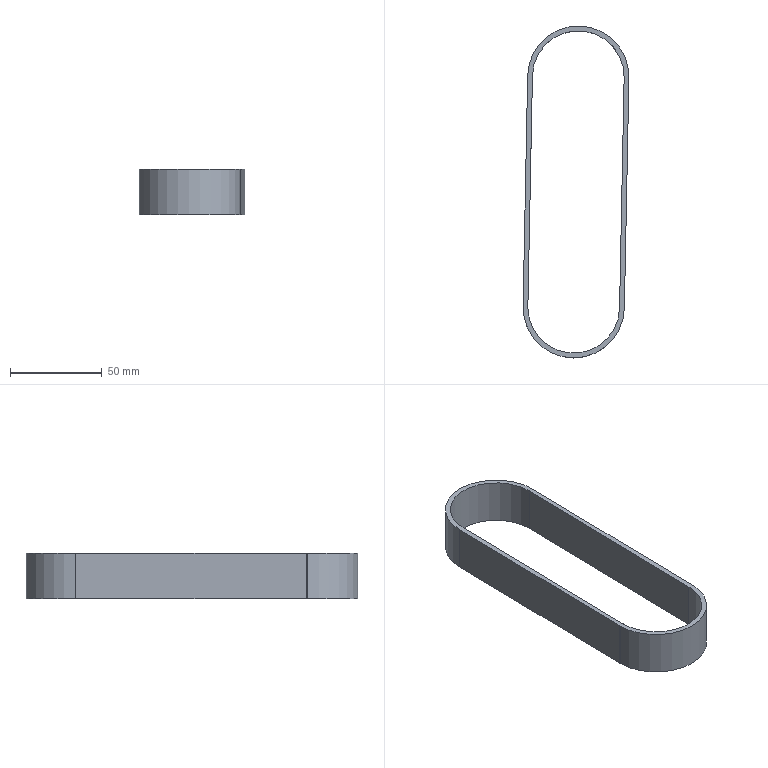Part | STEP file | Belt 2-3^ double-tube high-torque assembly | 1 solid | 12 faces | box 57.84 x 181.34 x 25 mm | volume 27358 mm3 | cylinder 6 | plane 6 | commonest cylinder face diameters 50.1 x3 55.34 x3
STEP:
#1=CARTESIAN_POINT('',(0.,0.,0.));
#2=DIRECTION('',(0.,0.,1.));
#3=DIRECTION('',(1.,0.,0.));
#4=AXIS2_PLACEMENT_3D('',#1,#2,#3);
#5=CARTESIAN_POINT('',(-25.045,0.4969,25.));
#6=VERTEX_POINT('',#5);
#7=CARTESIAN_POINT('',(-25.045,0.4969,0.));
#8=VERTEX_POINT('',#7);
#9=CARTESIAN_POINT('',(-25.045,0.4969,25.));
#10=DIRECTION('',(0.,0.,-1.));
#11=VECTOR('',#10,1.);
#12=LINE('',#9,#11);
#13=CARTESIAN_POINT('',(0.,0.,25.));
#14=DIRECTION('',(0.,0.,-1.));
#15=DIRECTION('',(-1.,0.,0.));
#16=AXIS2_PLACEMENT_3D('',#13,#14,#15);
#17=CYLINDRICAL_SURFACE('',#16,25.05);
#18=CARTESIAN_POINT('',(0.01984,0.));
#19=DIRECTION('',(0.,1.));
#20=VECTOR('',#19,1.);
#21=LINE('',#18,#20);
#22=(GEOMETRIC_REPRESENTATION_CONTEXT(2)PARAMETRIC_REPRESENTATION_CONTEXT()REPRESENTATION_CONTEXT('',''));
#23=DEFINITIONAL_REPRESENTATION('',(#21),#22);
#24=PCURVE('',#17,#23);
#25=CARTESIAN_POINT('',(-25.045,0.4969,25.));
#26=DIRECTION('',(-0.9998,0.01984,0.));
#27=DIRECTION('',(-0.01984,-0.9998,0.));
#28=AXIS2_PLACEMENT_3D('',#25,#26,#27);
#29=PLANE('',#28);
#30=CARTESIAN_POINT('',(0.,0.));
#31=DIRECTION('',(0.,-1.));
#32=VECTOR('',#31,1.);
#33=LINE('',#30,#32);
#34=(GEOMETRIC_REPRESENTATION_CONTEXT(2)PARAMETRIC_REPRESENTATION_CONTEXT()REPRESENTATION_CONTEXT('',''));
#35=DEFINITIONAL_REPRESENTATION('',(#33),#34);
#36=PCURVE('',#29,#35);
#37=SURFACE_CURVE('',#12,(#24,#36),.PCURVE_S1.);
#38=EDGE_CURVE('',#6,#8,#37,.T.);
#39=ORIENTED_EDGE('',*,*,#38,.T.);
#40=CARTESIAN_POINT('',(-25.05,0.,0.));
#41=VERTEX_POINT('',#40);
#42=CARTESIAN_POINT('',(0.,0.,0.));
#43=DIRECTION('',(0.,0.,-1.));
#44=DIRECTION('',(-1.,0.,0.));
#45=AXIS2_PLACEMENT_3D('',#42,#43,#44);
#46=CIRCLE('',#45,25.05);
#47=CARTESIAN_POINT('',(0.,25.));
#48=DIRECTION('',(1.,0.));
#49=VECTOR('',#48,1.);
#50=LINE('',#47,#49);
#51=(GEOMETRIC_REPRESENTATION_CONTEXT(2)PARAMETRIC_REPRESENTATION_CONTEXT()REPRESENTATION_CONTEXT('',''));
#52=DEFINITIONAL_REPRESENTATION('',(#50),#51);
#53=PCURVE('',#17,#52);
#54=CARTESIAN_POINT('',(2.5,126.,0.));
#55=DIRECTION('',(0.,0.,-1.));
#56=DIRECTION('',(-1.,0.,0.));
#57=AXIS2_PLACEMENT_3D('',#54,#55,#56);
#58=PLANE('',#57);
#59=CARTESIAN_POINT('',(2.5,-126.));
#60=DIRECTION('',(1.,0.));
#61=AXIS2_PLACEMENT_2D('',#59,#60);
#62=CIRCLE('',#61,25.05);
#63=(GEOMETRIC_REPRESENTATION_CONTEXT(2)PARAMETRIC_REPRESENTATION_CONTEXT()REPRESENTATION_CONTEXT('',''));
#64=DEFINITIONAL_REPRESENTATION('',(#62),#63);
#65=PCURVE('',#58,#64);
#66=SURFACE_CURVE('',#46,(#53,#65),.PCURVE_S1.);
#67=EDGE_CURVE('',#41,#8,#66,.T.);
#68=ORIENTED_EDGE('',*,*,#67,.F.);
#69=CARTESIAN_POINT('',(-25.05,0.,25.));
#70=VERTEX_POINT('',#69);
#71=CARTESIAN_POINT('',(-25.05,0.,25.));
#72=DIRECTION('',(0.,0.,-1.));
#73=VECTOR('',#72,1.);
#74=LINE('',#71,#73);
#75=CARTESIAN_POINT('',(0.,0.));
#76=DIRECTION('',(0.,1.));
#77=VECTOR('',#76,1.);
#78=LINE('',#75,#77);
#79=(GEOMETRIC_REPRESENTATION_CONTEXT(2)PARAMETRIC_REPRESENTATION_CONTEXT()REPRESENTATION_CONTEXT('',''));
#80=DEFINITIONAL_REPRESENTATION('',(#78),#79);
#81=PCURVE('',#17,#80);
#82=CARTESIAN_POINT('',(0.,0.,25.));
#83=DIRECTION('',(0.,0.,-1.));
#84=DIRECTION('',(-1.,0.,0.));
#85=AXIS2_PLACEMENT_3D('',#82,#83,#84);
#86=CYLINDRICAL_SURFACE('',#85,25.05);
#87=CARTESIAN_POINT('',(6.283,0.));
#88=DIRECTION('',(0.,1.));
#89=VECTOR('',#88,1.);
#90=LINE('',#87,#89);
#91=(GEOMETRIC_REPRESENTATION_CONTEXT(2)PARAMETRIC_REPRESENTATION_CONTEXT()REPRESENTATION_CONTEXT('',''));
#92=DEFINITIONAL_REPRESENTATION('',(#90),#91);
#93=PCURVE('',#86,#92);
#94=SURFACE_CURVE('',#74,(#81,#93),.PCURVE_S1.);
#95=EDGE_CURVE('',#70,#41,#94,.T.);
#96=ORIENTED_EDGE('',*,*,#95,.F.);
#97=CARTESIAN_POINT('',(0.,0.,25.));
#98=DIRECTION('',(0.,0.,-1.));
#99=DIRECTION('',(-1.,0.,0.));
#100=AXIS2_PLACEMENT_3D('',#97,#98,#99);
#101=CIRCLE('',#100,25.05);
#102=CARTESIAN_POINT('',(0.,0.));
#103=DIRECTION('',(1.,0.));
#104=VECTOR('',#103,1.);
#105=LINE('',#102,#104);
#106=(GEOMETRIC_REPRESENTATION_CONTEXT(2)PARAMETRIC_REPRESENTATION_CONTEXT()REPRESENTATION_CONTEXT('',''));
#107=DEFINITIONAL_REPRESENTATION('',(#105),#106);
#108=PCURVE('',#17,#107);
#109=CARTESIAN_POINT('',(2.5,126.,25.));
#110=DIRECTION('',(0.,0.,-1.));
#111=DIRECTION('',(-1.,0.,0.));
#112=AXIS2_PLACEMENT_3D('',#109,#110,#111);
#113=PLANE('',#112);
#114=CARTESIAN_POINT('',(2.5,-126.));
#115=DIRECTION('',(1.,0.));
#116=AXIS2_PLACEMENT_2D('',#114,#115);
#117=CIRCLE('',#116,25.05);
#118=(GEOMETRIC_REPRESENTATION_CONTEXT(2)PARAMETRIC_REPRESENTATION_CONTEXT()REPRESENTATION_CONTEXT('',''));
#119=DEFINITIONAL_REPRESENTATION('',(#117),#118);
#120=PCURVE('',#113,#119);
#121=SURFACE_CURVE('',#101,(#108,#120),.PCURVE_S1.);
#122=EDGE_CURVE('',#70,#6,#121,.T.);
#123=ORIENTED_EDGE('',*,*,#122,.T.);
#124=EDGE_LOOP('',(#39,#68,#96,#123));
#125=FACE_BOUND('',#124,.F.);
#126=ADVANCED_FACE('',(#125),#17,.F.);
#127=CARTESIAN_POINT('',(27.665,-0.5489,25.));
#128=VERTEX_POINT('',#127);
#129=CARTESIAN_POINT('',(-27.67,0.,25.));
#130=VERTEX_POINT('',#129);
#131=CARTESIAN_POINT('',(0.,0.,25.));
#132=DIRECTION('',(0.,0.,-1.));
#133=DIRECTION('',(-1.,0.,0.));
#134=AXIS2_PLACEMENT_3D('',#131,#132,#133);
#135=CIRCLE('',#134,27.67);
#136=CARTESIAN_POINT('',(0.,0.,25.));
#137=DIRECTION('',(0.,0.,-1.));
#138=DIRECTION('',(-1.,0.,0.));
#139=AXIS2_PLACEMENT_3D('',#136,#137,#138);
#140=CYLINDRICAL_SURFACE('',#139,27.67);
#141=CARTESIAN_POINT('',(0.,0.));
#142=DIRECTION('',(1.,0.));
#143=VECTOR('',#142,1.);
#144=LINE('',#141,#143);
#145=(GEOMETRIC_REPRESENTATION_CONTEXT(2)PARAMETRIC_REPRESENTATION_CONTEXT()REPRESENTATION_CONTEXT('',''));
#146=DEFINITIONAL_REPRESENTATION('',(#144),#145);
#147=PCURVE('',#140,#146);
#148=CARTESIAN_POINT('',(2.5,-126.));
#149=DIRECTION('',(1.,0.));
#150=AXIS2_PLACEMENT_2D('',#148,#149);
#151=CIRCLE('',#150,27.67);
#152=(GEOMETRIC_REPRESENTATION_CONTEXT(2)PARAMETRIC_REPRESENTATION_CONTEXT()REPRESENTATION_CONTEXT('',''));
#153=DEFINITIONAL_REPRESENTATION('',(#151),#152);
#154=PCURVE('',#113,#153);
#155=SURFACE_CURVE('',#135,(#147,#154),.PCURVE_S1.);
#156=EDGE_CURVE('',#128,#130,#155,.T.);
#157=ORIENTED_EDGE('',*,*,#156,.T.);
#158=CARTESIAN_POINT('',(-27.67,0.,0.));
#159=VERTEX_POINT('',#158);
#160=CARTESIAN_POINT('',(-27.67,0.,25.));
#161=DIRECTION('',(0.,0.,-1.));
#162=VECTOR('',#161,1.);
#163=LINE('',#160,#162);
#164=CARTESIAN_POINT('',(6.283,0.));
#165=DIRECTION('',(0.,1.));
#166=VECTOR('',#165,1.);
#167=LINE('',#164,#166);
#168=(GEOMETRIC_REPRESENTATION_CONTEXT(2)PARAMETRIC_REPRESENTATION_CONTEXT()REPRESENTATION_CONTEXT('',''));
#169=DEFINITIONAL_REPRESENTATION('',(#167),#168);
#170=PCURVE('',#140,#169);
#171=CARTESIAN_POINT('',(0.,0.,25.));
#172=DIRECTION('',(0.,0.,-1.));
#173=DIRECTION('',(-1.,0.,0.));
#174=AXIS2_PLACEMENT_3D('',#171,#172,#173);
#175=CYLINDRICAL_SURFACE('',#174,27.67);
#176=CARTESIAN_POINT('',(0.,0.));
#177=DIRECTION('',(0.,1.));
#178=VECTOR('',#177,1.);
#179=LINE('',#176,#178);
#180=(GEOMETRIC_REPRESENTATION_CONTEXT(2)PARAMETRIC_REPRESENTATION_CONTEXT()REPRESENTATION_CONTEXT('',''));
#181=DEFINITIONAL_REPRESENTATION('',(#179),#180);
#182=PCURVE('',#175,#181);
#183=SURFACE_CURVE('',#163,(#170,#182),.PCURVE_S1.);
#184=EDGE_CURVE('',#130,#159,#183,.T.);
#185=ORIENTED_EDGE('',*,*,#184,.T.);
#186=CARTESIAN_POINT('',(27.665,-0.5489,0.));
#187=VERTEX_POINT('',#186);
#188=CARTESIAN_POINT('',(0.,0.,0.));
#189=DIRECTION('',(0.,0.,-1.));
#190=DIRECTION('',(-1.,0.,0.));
#191=AXIS2_PLACEMENT_3D('',#188,#189,#190);
#192=CIRCLE('',#191,27.67);
#193=CARTESIAN_POINT('',(0.,25.));
#194=DIRECTION('',(1.,0.));
#195=VECTOR('',#194,1.);
#196=LINE('',#193,#195);
#197=(GEOMETRIC_REPRESENTATION_CONTEXT(2)PARAMETRIC_REPRESENTATION_CONTEXT()REPRESENTATION_CONTEXT('',''));
#198=DEFINITIONAL_REPRESENTATION('',(#196),#197);
#199=PCURVE('',#140,#198);
#200=CARTESIAN_POINT('',(2.5,-126.));
#201=DIRECTION('',(1.,0.));
#202=AXIS2_PLACEMENT_2D('',#200,#201);
#203=CIRCLE('',#202,27.67);
#204=(GEOMETRIC_REPRESENTATION_CONTEXT(2)PARAMETRIC_REPRESENTATION_CONTEXT()REPRESENTATION_CONTEXT('',''));
#205=DEFINITIONAL_REPRESENTATION('',(#203),#204);
#206=PCURVE('',#58,#205);
#207=SURFACE_CURVE('',#192,(#199,#206),.PCURVE_S1.);
#208=EDGE_CURVE('',#187,#159,#207,.T.);
#209=ORIENTED_EDGE('',*,*,#208,.F.);
#210=CARTESIAN_POINT('',(27.665,-0.5489,25.));
#211=DIRECTION('',(0.,0.,-1.));
#212=VECTOR('',#211,1.);
#213=LINE('',#210,#212);
#214=CARTESIAN_POINT('',(3.161,0.));
#215=DIRECTION('',(0.,1.));
#216=VECTOR('',#215,1.);
#217=LINE('',#214,#216);
#218=(GEOMETRIC_REPRESENTATION_CONTEXT(2)PARAMETRIC_REPRESENTATION_CONTEXT()REPRESENTATION_CONTEXT('',''));
#219=DEFINITIONAL_REPRESENTATION('',(#217),#218);
#220=PCURVE('',#140,#219);
#221=CARTESIAN_POINT('',(30.165,125.451,25.));
#222=DIRECTION('',(0.9998,-0.01984,0.));
#223=DIRECTION('',(0.01984,0.9998,0.));
#224=AXIS2_PLACEMENT_3D('',#221,#222,#223);
#225=PLANE('',#224);
#226=CARTESIAN_POINT('',(-126.025,0.));
#227=DIRECTION('',(0.,-1.));
#228=VECTOR('',#227,1.);
#229=LINE('',#226,#228);
#230=(GEOMETRIC_REPRESENTATION_CONTEXT(2)PARAMETRIC_REPRESENTATION_CONTEXT()REPRESENTATION_CONTEXT('',''));
#231=DEFINITIONAL_REPRESENTATION('',(#229),#230);
#232=PCURVE('',#225,#231);
#233=SURFACE_CURVE('',#213,(#220,#232),.PCURVE_S1.);
#234=EDGE_CURVE('',#128,#187,#233,.T.);
#235=ORIENTED_EDGE('',*,*,#234,.F.);
#236=EDGE_LOOP('',(#157,#185,#209,#235));
#237=FACE_BOUND('',#236,.T.);
#238=ADVANCED_FACE('',(#237),#140,.T.);
#239=CARTESIAN_POINT('',(-25.165,126.549,0.));
#240=VERTEX_POINT('',#239);
#241=CARTESIAN_POINT('',(30.165,125.451,0.));
#242=VERTEX_POINT('',#241);
#243=CARTESIAN_POINT('',(2.5,126.,0.));
#244=DIRECTION('',(0.,0.,-1.));
#245=DIRECTION('',(-1.,0.,0.));
#246=AXIS2_PLACEMENT_3D('',#243,#244,#245);
#247=CIRCLE('',#246,27.67);
#248=CARTESIAN_POINT('',(2.5,126.,25.));
#249=DIRECTION('',(0.,0.,-1.));
#250=DIRECTION('',(-1.,0.,0.));
#251=AXIS2_PLACEMENT_3D('',#248,#249,#250);
#252=CYLINDRICAL_SURFACE('',#251,27.67);
#253=CARTESIAN_POINT('',(0.,25.));
#254=DIRECTION('',(1.,0.));
#255=VECTOR('',#254,1.);
#256=LINE('',#253,#255);
#257=(GEOMETRIC_REPRESENTATION_CONTEXT(2)PARAMETRIC_REPRESENTATION_CONTEXT()REPRESENTATION_CONTEXT('',''));
#258=DEFINITIONAL_REPRESENTATION('',(#256),#257);
#259=PCURVE('',#252,#258);
#260=CARTESIAN_POINT('',(0.,0.));
#261=DIRECTION('',(1.,0.));
#262=AXIS2_PLACEMENT_2D('',#260,#261);
#263=CIRCLE('',#262,27.67);
#264=(GEOMETRIC_REPRESENTATION_CONTEXT(2)PARAMETRIC_REPRESENTATION_CONTEXT()REPRESENTATION_CONTEXT('',''));
#265=DEFINITIONAL_REPRESENTATION('',(#263),#264);
#266=PCURVE('',#58,#265);
#267=SURFACE_CURVE('',#247,(#259,#266),.PCURVE_S1.);
#268=EDGE_CURVE('',#240,#242,#267,.T.);
#269=ORIENTED_EDGE('',*,*,#268,.F.);
#270=CARTESIAN_POINT('',(-25.165,126.549,25.));
#271=VERTEX_POINT('',#270);
#272=CARTESIAN_POINT('',(-25.165,126.549,25.));
#273=DIRECTION('',(0.,0.,-1.));
#274=VECTOR('',#273,1.);
#275=LINE('',#272,#274);
#276=CARTESIAN_POINT('',(0.01984,0.));
#277=DIRECTION('',(0.,1.));
#278=VECTOR('',#277,1.);
#279=LINE('',#276,#278);
#280=(GEOMETRIC_REPRESENTATION_CONTEXT(2)PARAMETRIC_REPRESENTATION_CONTEXT()REPRESENTATION_CONTEXT('',''));
#281=DEFINITIONAL_REPRESENTATION('',(#279),#280);
#282=PCURVE('',#252,#281);
#283=CARTESIAN_POINT('',(-25.165,126.549,25.));
#284=DIRECTION('',(-0.9998,0.01984,0.));
#285=DIRECTION('',(-0.01984,-0.9998,0.));
#286=AXIS2_PLACEMENT_3D('',#283,#284,#285);
#287=PLANE('',#286);
#288=CARTESIAN_POINT('',(0.,0.));
#289=DIRECTION('',(0.,-1.));
#290=VECTOR('',#289,1.);
#291=LINE('',#288,#290);
#292=(GEOMETRIC_REPRESENTATION_CONTEXT(2)PARAMETRIC_REPRESENTATION_CONTEXT()REPRESENTATION_CONTEXT('',''));
#293=DEFINITIONAL_REPRESENTATION('',(#291),#292);
#294=PCURVE('',#287,#293);
#295=SURFACE_CURVE('',#275,(#282,#294),.PCURVE_S1.);
#296=EDGE_CURVE('',#271,#240,#295,.T.);
#297=ORIENTED_EDGE('',*,*,#296,.F.);
#298=CARTESIAN_POINT('',(30.165,125.451,25.));
#299=VERTEX_POINT('',#298);
#300=CARTESIAN_POINT('',(2.5,126.,25.));
#301=DIRECTION('',(0.,0.,-1.));
#302=DIRECTION('',(-1.,0.,0.));
#303=AXIS2_PLACEMENT_3D('',#300,#301,#302);
#304=CIRCLE('',#303,27.67);
#305=CARTESIAN_POINT('',(0.,0.));
#306=DIRECTION('',(1.,0.));
#307=VECTOR('',#306,1.);
#308=LINE('',#305,#307);
#309=(GEOMETRIC_REPRESENTATION_CONTEXT(2)PARAMETRIC_REPRESENTATION_CONTEXT()REPRESENTATION_CONTEXT('',''));
#310=DEFINITIONAL_REPRESENTATION('',(#308),#309);
#311=PCURVE('',#252,#310);
#312=CARTESIAN_POINT('',(0.,0.));
#313=DIRECTION('',(1.,0.));
#314=AXIS2_PLACEMENT_2D('',#312,#313);
#315=CIRCLE('',#314,27.67);
#316=(GEOMETRIC_REPRESENTATION_CONTEXT(2)PARAMETRIC_REPRESENTATION_CONTEXT()REPRESENTATION_CONTEXT('',''));
#317=DEFINITIONAL_REPRESENTATION('',(#315),#316);
#318=PCURVE('',#113,#317);
#319=SURFACE_CURVE('',#304,(#311,#318),.PCURVE_S1.);
#320=EDGE_CURVE('',#271,#299,#319,.T.);
#321=ORIENTED_EDGE('',*,*,#320,.T.);
#322=CARTESIAN_POINT('',(30.165,125.451,25.));
#323=DIRECTION('',(0.,0.,-1.));
#324=VECTOR('',#323,1.);
#325=LINE('',#322,#324);
#326=CARTESIAN_POINT('',(3.161,0.));
#327=DIRECTION('',(0.,1.));
#328=VECTOR('',#327,1.);
#329=LINE('',#326,#328);
#330=(GEOMETRIC_REPRESENTATION_CONTEXT(2)PARAMETRIC_REPRESENTATION_CONTEXT()REPRESENTATION_CONTEXT('',''));
#331=DEFINITIONAL_REPRESENTATION('',(#329),#330);
#332=PCURVE('',#252,#331);
#333=CARTESIAN_POINT('',(0.,0.));
#334=DIRECTION('',(0.,-1.));
#335=VECTOR('',#334,1.);
#336=LINE('',#333,#335);
#337=(GEOMETRIC_REPRESENTATION_CONTEXT(2)PARAMETRIC_REPRESENTATION_CONTEXT()REPRESENTATION_CONTEXT('',''));
#338=DEFINITIONAL_REPRESENTATION('',(#336),#337);
#339=PCURVE('',#225,#338);
#340=SURFACE_CURVE('',#325,(#332,#339),.PCURVE_S1.);
#341=EDGE_CURVE('',#299,#242,#340,.T.);
#342=ORIENTED_EDGE('',*,*,#341,.T.);
#343=EDGE_LOOP('',(#269,#297,#321,#342));
#344=FACE_BOUND('',#343,.T.);
#345=ADVANCED_FACE('',(#344),#252,.T.);
#346=CARTESIAN_POINT('',(-27.665,0.5489,0.));
#347=VERTEX_POINT('',#346);
#348=CARTESIAN_POINT('',(-25.165,126.549,0.));
#349=DIRECTION('',(0.01984,0.9998,0.));
#350=VECTOR('',#349,1.);
#351=LINE('',#348,#350);
#352=CARTESIAN_POINT('',(0.,-25.));
#353=DIRECTION('',(-1.,0.));
#354=VECTOR('',#353,1.);
#355=LINE('',#352,#354);
#356=(GEOMETRIC_REPRESENTATION_CONTEXT(2)PARAMETRIC_REPRESENTATION_CONTEXT()REPRESENTATION_CONTEXT('',''));
#357=DEFINITIONAL_REPRESENTATION('',(#355),#356);
#358=PCURVE('',#287,#357);
#359=CARTESIAN_POINT('',(27.665,0.5489));
#360=DIRECTION('',(-0.01984,0.9998));
#361=VECTOR('',#360,1.);
#362=LINE('',#359,#361);
#363=(GEOMETRIC_REPRESENTATION_CONTEXT(2)PARAMETRIC_REPRESENTATION_CONTEXT()REPRESENTATION_CONTEXT('',''));
#364=DEFINITIONAL_REPRESENTATION('',(#362),#363);
#365=PCURVE('',#58,#364);
#366=SURFACE_CURVE('',#351,(#358,#365),.PCURVE_S1.);
#367=EDGE_CURVE('',#347,#240,#366,.T.);
#368=ORIENTED_EDGE('',*,*,#367,.F.);
#369=CARTESIAN_POINT('',(-27.665,0.5489,25.));
#370=VERTEX_POINT('',#369);
#371=CARTESIAN_POINT('',(-27.665,0.5489,25.));
#372=DIRECTION('',(0.,0.,-1.));
#373=VECTOR('',#372,1.);
#374=LINE('',#371,#373);
#375=CARTESIAN_POINT('',(126.025,0.));
#376=DIRECTION('',(0.,-1.));
#377=VECTOR('',#376,1.);
#378=LINE('',#375,#377);
#379=(GEOMETRIC_REPRESENTATION_CONTEXT(2)PARAMETRIC_REPRESENTATION_CONTEXT()REPRESENTATION_CONTEXT('',''));
#380=DEFINITIONAL_REPRESENTATION('',(#378),#379);
#381=PCURVE('',#287,#380);
#382=CARTESIAN_POINT('',(0.01984,0.));
#383=DIRECTION('',(0.,1.));
#384=VECTOR('',#383,1.);
#385=LINE('',#382,#384);
#386=(GEOMETRIC_REPRESENTATION_CONTEXT(2)PARAMETRIC_REPRESENTATION_CONTEXT()REPRESENTATION_CONTEXT('',''));
#387=DEFINITIONAL_REPRESENTATION('',(#385),#386);
#388=PCURVE('',#175,#387);
#389=SURFACE_CURVE('',#374,(#381,#388),.PCURVE_S1.);
#390=EDGE_CURVE('',#370,#347,#389,.T.);
#391=ORIENTED_EDGE('',*,*,#390,.F.);
#392=CARTESIAN_POINT('',(-25.165,126.549,25.));
#393=DIRECTION('',(0.01984,0.9998,0.));
#394=VECTOR('',#393,1.);
#395=LINE('',#392,#394);
#396=CARTESIAN_POINT('',(0.,0.));
#397=DIRECTION('',(-1.,0.));
#398=VECTOR('',#397,1.);
#399=LINE('',#396,#398);
#400=(GEOMETRIC_REPRESENTATION_CONTEXT(2)PARAMETRIC_REPRESENTATION_CONTEXT()REPRESENTATION_CONTEXT('',''));
#401=DEFINITIONAL_REPRESENTATION('',(#399),#400);
#402=PCURVE('',#287,#401);
#403=CARTESIAN_POINT('',(27.665,0.5489));
#404=DIRECTION('',(-0.01984,0.9998));
#405=VECTOR('',#404,1.);
#406=LINE('',#403,#405);
#407=(GEOMETRIC_REPRESENTATION_CONTEXT(2)PARAMETRIC_REPRESENTATION_CONTEXT()REPRESENTATION_CONTEXT('',''));
#408=DEFINITIONAL_REPRESENTATION('',(#406),#407);
#409=PCURVE('',#113,#408);
#410=SURFACE_CURVE('',#395,(#402,#409),.PCURVE_S1.);
#411=EDGE_CURVE('',#370,#271,#410,.T.);
#412=ORIENTED_EDGE('',*,*,#411,.T.);
#413=ORIENTED_EDGE('',*,*,#296,.T.);
#414=EDGE_LOOP('',(#368,#391,#412,#413));
#415=FACE_BOUND('',#414,.T.);
#416=ADVANCED_FACE('',(#415),#287,.T.);
#417=ORIENTED_EDGE('',*,*,#184,.F.);
#418=CARTESIAN_POINT('',(0.,0.,25.));
#419=DIRECTION('',(0.,0.,-1.));
#420=DIRECTION('',(-1.,0.,0.));
#421=AXIS2_PLACEMENT_3D('',#418,#419,#420);
#422=CIRCLE('',#421,27.67);
#423=CARTESIAN_POINT('',(0.,0.));
#424=DIRECTION('',(1.,0.));
#425=VECTOR('',#424,1.);
#426=LINE('',#423,#425);
#427=(GEOMETRIC_REPRESENTATION_CONTEXT(2)PARAMETRIC_REPRESENTATION_CONTEXT()REPRESENTATION_CONTEXT('',''));
#428=DEFINITIONAL_REPRESENTATION('',(#426),#427);
#429=PCURVE('',#175,#428);
#430=CARTESIAN_POINT('',(2.5,-126.));
#431=DIRECTION('',(1.,0.));
#432=AXIS2_PLACEMENT_2D('',#430,#431);
#433=CIRCLE('',#432,27.67);
#434=(GEOMETRIC_REPRESENTATION_CONTEXT(2)PARAMETRIC_REPRESENTATION_CONTEXT()REPRESENTATION_CONTEXT('',''));
#435=DEFINITIONAL_REPRESENTATION('',(#433),#434);
#436=PCURVE('',#113,#435);
#437=SURFACE_CURVE('',#422,(#429,#436),.PCURVE_S1.);
#438=EDGE_CURVE('',#130,#370,#437,.T.);
#439=ORIENTED_EDGE('',*,*,#438,.T.);
#440=ORIENTED_EDGE('',*,*,#390,.T.);
#441=CARTESIAN_POINT('',(0.,0.,0.));
#442=DIRECTION('',(0.,0.,-1.));
#443=DIRECTION('',(-1.,0.,0.));
#444=AXIS2_PLACEMENT_3D('',#441,#442,#443);
#445=CIRCLE('',#444,27.67);
#446=CARTESIAN_POINT('',(0.,25.));
#447=DIRECTION('',(1.,0.));
#448=VECTOR('',#447,1.);
#449=LINE('',#446,#448);
#450=(GEOMETRIC_REPRESENTATION_CONTEXT(2)PARAMETRIC_REPRESENTATION_CONTEXT()REPRESENTATION_CONTEXT('',''));
#451=DEFINITIONAL_REPRESENTATION('',(#449),#450);
#452=PCURVE('',#175,#451);
#453=CARTESIAN_POINT('',(2.5,-126.));
#454=DIRECTION('',(1.,0.));
#455=AXIS2_PLACEMENT_2D('',#453,#454);
#456=CIRCLE('',#455,27.67);
#457=(GEOMETRIC_REPRESENTATION_CONTEXT(2)PARAMETRIC_REPRESENTATION_CONTEXT()REPRESENTATION_CONTEXT('',''));
#458=DEFINITIONAL_REPRESENTATION('',(#456),#457);
#459=PCURVE('',#58,#458);
#460=SURFACE_CURVE('',#445,(#452,#459),.PCURVE_S1.);
#461=EDGE_CURVE('',#159,#347,#460,.T.);
#462=ORIENTED_EDGE('',*,*,#461,.F.);
#463=EDGE_LOOP('',(#417,#439,#440,#462));
#464=FACE_BOUND('',#463,.T.);
#465=ADVANCED_FACE('',(#464),#175,.T.);
#466=CARTESIAN_POINT('',(30.165,125.451,0.));
#467=DIRECTION('',(-0.01984,-0.9998,0.));
#468=VECTOR('',#467,1.);
#469=LINE('',#466,#468);
#470=CARTESIAN_POINT('',(0.,-25.));
#471=DIRECTION('',(-1.,0.));
#472=VECTOR('',#471,1.);
#473=LINE('',#470,#472);
#474=(GEOMETRIC_REPRESENTATION_CONTEXT(2)PARAMETRIC_REPRESENTATION_CONTEXT()REPRESENTATION_CONTEXT('',''));
#475=DEFINITIONAL_REPRESENTATION('',(#473),#474);
#476=PCURVE('',#225,#475);
#477=CARTESIAN_POINT('',(-27.665,-0.5489));
#478=DIRECTION('',(0.01984,-0.9998));
#479=VECTOR('',#478,1.);
#480=LINE('',#477,#479);
#481=(GEOMETRIC_REPRESENTATION_CONTEXT(2)PARAMETRIC_REPRESENTATION_CONTEXT()REPRESENTATION_CONTEXT('',''));
#482=DEFINITIONAL_REPRESENTATION('',(#480),#481);
#483=PCURVE('',#58,#482);
#484=SURFACE_CURVE('',#469,(#476,#483),.PCURVE_S1.);
#485=EDGE_CURVE('',#242,#187,#484,.T.);
#486=ORIENTED_EDGE('',*,*,#485,.F.);
#487=ORIENTED_EDGE('',*,*,#341,.F.);
#488=CARTESIAN_POINT('',(30.165,125.451,25.));
#489=DIRECTION('',(-0.01984,-0.9998,0.));
#490=VECTOR('',#489,1.);
#491=LINE('',#488,#490);
#492=CARTESIAN_POINT('',(0.,0.));
#493=DIRECTION('',(-1.,0.));
#494=VECTOR('',#493,1.);
#495=LINE('',#492,#494);
#496=(GEOMETRIC_REPRESENTATION_CONTEXT(2)PARAMETRIC_REPRESENTATION_CONTEXT()REPRESENTATION_CONTEXT('',''));
#497=DEFINITIONAL_REPRESENTATION('',(#495),#496);
#498=PCURVE('',#225,#497);
#499=CARTESIAN_POINT('',(-27.665,-0.5489));
#500=DIRECTION('',(0.01984,-0.9998));
#501=VECTOR('',#500,1.);
#502=LINE('',#499,#501);
#503=(GEOMETRIC_REPRESENTATION_CONTEXT(2)PARAMETRIC_REPRESENTATION_CONTEXT()REPRESENTATION_CONTEXT('',''));
#504=DEFINITIONAL_REPRESENTATION('',(#502),#503);
#505=PCURVE('',#113,#504);
#506=SURFACE_CURVE('',#491,(#498,#505),.PCURVE_S1.);
#507=EDGE_CURVE('',#299,#128,#506,.T.);
#508=ORIENTED_EDGE('',*,*,#507,.T.);
#509=ORIENTED_EDGE('',*,*,#234,.T.);
#510=EDGE_LOOP('',(#486,#487,#508,#509));
#511=FACE_BOUND('',#510,.T.);
#512=ADVANCED_FACE('',(#511),#225,.T.);
#513=CARTESIAN_POINT('',(-22.545,126.497,25.));
#514=VERTEX_POINT('',#513);
#515=CARTESIAN_POINT('',(-25.045,0.4969,25.));
#516=DIRECTION('',(0.01984,0.9998,0.));
#517=VECTOR('',#516,1.);
#518=LINE('',#515,#517);
#519=CARTESIAN_POINT('',(27.545,-125.503));
#520=DIRECTION('',(-0.01984,0.9998));
#521=VECTOR('',#520,1.);
#522=LINE('',#519,#521);
#523=(GEOMETRIC_REPRESENTATION_CONTEXT(2)PARAMETRIC_REPRESENTATION_CONTEXT()REPRESENTATION_CONTEXT('',''));
#524=DEFINITIONAL_REPRESENTATION('',(#522),#523);
#525=PCURVE('',#113,#524);
#526=CARTESIAN_POINT('',(0.,0.));
#527=DIRECTION('',(-1.,0.));
#528=VECTOR('',#527,1.);
#529=LINE('',#526,#528);
#530=(GEOMETRIC_REPRESENTATION_CONTEXT(2)PARAMETRIC_REPRESENTATION_CONTEXT()REPRESENTATION_CONTEXT('',''));
#531=DEFINITIONAL_REPRESENTATION('',(#529),#530);
#532=PCURVE('',#29,#531);
#533=SURFACE_CURVE('',#518,(#525,#532),.PCURVE_S1.);
#534=EDGE_CURVE('',#6,#514,#533,.T.);
#535=ORIENTED_EDGE('',*,*,#534,.T.);
#536=CARTESIAN_POINT('',(27.545,125.503,25.));
#537=VERTEX_POINT('',#536);
#538=CARTESIAN_POINT('',(2.5,126.,25.));
#539=DIRECTION('',(0.,0.,-1.));
#540=DIRECTION('',(-1.,0.,0.));
#541=AXIS2_PLACEMENT_3D('',#538,#539,#540);
#542=CIRCLE('',#541,25.05);
#543=CARTESIAN_POINT('',(0.,0.));
#544=DIRECTION('',(1.,0.));
#545=AXIS2_PLACEMENT_2D('',#543,#544);
#546=CIRCLE('',#545,25.05);
#547=(GEOMETRIC_REPRESENTATION_CONTEXT(2)PARAMETRIC_REPRESENTATION_CONTEXT()REPRESENTATION_CONTEXT('',''));
#548=DEFINITIONAL_REPRESENTATION('',(#546),#547);
#549=PCURVE('',#113,#548);
#550=CARTESIAN_POINT('',(2.5,126.,25.));
#551=DIRECTION('',(0.,0.,-1.));
#552=DIRECTION('',(-1.,0.,0.));
#553=AXIS2_PLACEMENT_3D('',#550,#551,#552);
#554=CYLINDRICAL_SURFACE('',#553,25.05);
#555=CARTESIAN_POINT('',(0.,0.));
#556=DIRECTION('',(1.,0.));
#557=VECTOR('',#556,1.);
#558=LINE('',#555,#557);
#559=(GEOMETRIC_REPRESENTATION_CONTEXT(2)PARAMETRIC_REPRESENTATION_CONTEXT()REPRESENTATION_CONTEXT('',''));
#560=DEFINITIONAL_REPRESENTATION('',(#558),#559);
#561=PCURVE('',#554,#560);
#562=SURFACE_CURVE('',#542,(#549,#561),.PCURVE_S1.);
#563=EDGE_CURVE('',#514,#537,#562,.T.);
#564=ORIENTED_EDGE('',*,*,#563,.T.);
#565=CARTESIAN_POINT('',(25.045,-0.4969,25.));
#566=VERTEX_POINT('',#565);
#567=CARTESIAN_POINT('',(27.545,125.503,25.));
#568=DIRECTION('',(-0.01984,-0.9998,0.));
#569=VECTOR('',#568,1.);
#570=LINE('',#567,#569);
#571=CARTESIAN_POINT('',(-25.045,-0.4969));
#572=DIRECTION('',(0.01984,-0.9998));
#573=VECTOR('',#572,1.);
#574=LINE('',#571,#573);
#575=(GEOMETRIC_REPRESENTATION_CONTEXT(2)PARAMETRIC_REPRESENTATION_CONTEXT()REPRESENTATION_CONTEXT('',''));
#576=DEFINITIONAL_REPRESENTATION('',(#574),#575);
#577=PCURVE('',#113,#576);
#578=CARTESIAN_POINT('',(27.545,125.503,25.));
#579=DIRECTION('',(0.9998,-0.01984,0.));
#580=DIRECTION('',(0.01984,0.9998,0.));
#581=AXIS2_PLACEMENT_3D('',#578,#579,#580);
#582=PLANE('',#581);
#583=CARTESIAN_POINT('',(0.,0.));
#584=DIRECTION('',(-1.,0.));
#585=VECTOR('',#584,1.);
#586=LINE('',#583,#585);
#587=(GEOMETRIC_REPRESENTATION_CONTEXT(2)PARAMETRIC_REPRESENTATION_CONTEXT()REPRESENTATION_CONTEXT('',''));
#588=DEFINITIONAL_REPRESENTATION('',(#586),#587);
#589=PCURVE('',#582,#588);
#590=SURFACE_CURVE('',#570,(#577,#589),.PCURVE_S1.);
#591=EDGE_CURVE('',#537,#566,#590,.T.);
#592=ORIENTED_EDGE('',*,*,#591,.T.);
#593=CARTESIAN_POINT('',(0.,0.,25.));
#594=DIRECTION('',(0.,0.,-1.));
#595=DIRECTION('',(-1.,0.,0.));
#596=AXIS2_PLACEMENT_3D('',#593,#594,#595);
#597=CIRCLE('',#596,25.05);
#598=CARTESIAN_POINT('',(2.5,-126.));
#599=DIRECTION('',(1.,0.));
#600=AXIS2_PLACEMENT_2D('',#598,#599);
#601=CIRCLE('',#600,25.05);
#602=(GEOMETRIC_REPRESENTATION_CONTEXT(2)PARAMETRIC_REPRESENTATION_CONTEXT()REPRESENTATION_CONTEXT('',''));
#603=DEFINITIONAL_REPRESENTATION('',(#601),#602);
#604=PCURVE('',#113,#603);
#605=CARTESIAN_POINT('',(0.,0.));
#606=DIRECTION('',(1.,0.));
#607=VECTOR('',#606,1.);
#608=LINE('',#605,#607);
#609=(GEOMETRIC_REPRESENTATION_CONTEXT(2)PARAMETRIC_REPRESENTATION_CONTEXT()REPRESENTATION_CONTEXT('',''));
#610=DEFINITIONAL_REPRESENTATION('',(#608),#609);
#611=PCURVE('',#86,#610);
#612=SURFACE_CURVE('',#597,(#604,#611),.PCURVE_S1.);
#613=EDGE_CURVE('',#566,#70,#612,.T.);
#614=ORIENTED_EDGE('',*,*,#613,.T.);
#615=ORIENTED_EDGE('',*,*,#122,.T.);
#616=EDGE_LOOP('',(#535,#564,#592,#614,#615));
#617=FACE_BOUND('',#616,.T.);
#618=ORIENTED_EDGE('',*,*,#320,.F.);
#619=ORIENTED_EDGE('',*,*,#411,.F.);
#620=ORIENTED_EDGE('',*,*,#438,.F.);
#621=ORIENTED_EDGE('',*,*,#156,.F.);
#622=ORIENTED_EDGE('',*,*,#507,.F.);
#623=EDGE_LOOP('',(#618,#619,#620,#621,#622));
#624=FACE_BOUND('',#623,.T.);
#625=ADVANCED_FACE('',(#617,#624),#113,.F.);
#626=CARTESIAN_POINT('',(-22.545,126.497,0.));
#627=VERTEX_POINT('',#626);
#628=CARTESIAN_POINT('',(27.545,125.503,0.));
#629=VERTEX_POINT('',#628);
#630=CARTESIAN_POINT('',(2.5,126.,0.));
#631=DIRECTION('',(0.,0.,-1.));
#632=DIRECTION('',(-1.,0.,0.));
#633=AXIS2_PLACEMENT_3D('',#630,#631,#632);
#634=CIRCLE('',#633,25.05);
#635=CARTESIAN_POINT('',(0.,0.));
#636=DIRECTION('',(1.,0.));
#637=AXIS2_PLACEMENT_2D('',#635,#636);
#638=CIRCLE('',#637,25.05);
#639=(GEOMETRIC_REPRESENTATION_CONTEXT(2)PARAMETRIC_REPRESENTATION_CONTEXT()REPRESENTATION_CONTEXT('',''));
#640=DEFINITIONAL_REPRESENTATION('',(#638),#639);
#641=PCURVE('',#58,#640);
#642=CARTESIAN_POINT('',(0.,25.));
#643=DIRECTION('',(1.,0.));
#644=VECTOR('',#643,1.);
#645=LINE('',#642,#644);
#646=(GEOMETRIC_REPRESENTATION_CONTEXT(2)PARAMETRIC_REPRESENTATION_CONTEXT()REPRESENTATION_CONTEXT('',''));
#647=DEFINITIONAL_REPRESENTATION('',(#645),#646);
#648=PCURVE('',#554,#647);
#649=SURFACE_CURVE('',#634,(#641,#648),.PCURVE_S1.);
#650=EDGE_CURVE('',#627,#629,#649,.T.);
#651=ORIENTED_EDGE('',*,*,#650,.F.);
#652=CARTESIAN_POINT('',(-25.045,0.4969,0.));
#653=DIRECTION('',(0.01984,0.9998,0.));
#654=VECTOR('',#653,1.);
#655=LINE('',#652,#654);
#656=CARTESIAN_POINT('',(27.545,-125.503));
#657=DIRECTION('',(-0.01984,0.9998));
#658=VECTOR('',#657,1.);
#659=LINE('',#656,#658);
#660=(GEOMETRIC_REPRESENTATION_CONTEXT(2)PARAMETRIC_REPRESENTATION_CONTEXT()REPRESENTATION_CONTEXT('',''));
#661=DEFINITIONAL_REPRESENTATION('',(#659),#660);
#662=PCURVE('',#58,#661);
#663=CARTESIAN_POINT('',(0.,-25.));
#664=DIRECTION('',(-1.,0.));
#665=VECTOR('',#664,1.);
#666=LINE('',#663,#665);
#667=(GEOMETRIC_REPRESENTATION_CONTEXT(2)PARAMETRIC_REPRESENTATION_CONTEXT()REPRESENTATION_CONTEXT('',''));
#668=DEFINITIONAL_REPRESENTATION('',(#666),#667);
#669=PCURVE('',#29,#668);
#670=SURFACE_CURVE('',#655,(#662,#669),.PCURVE_S1.);
#671=EDGE_CURVE('',#8,#627,#670,.T.);
#672=ORIENTED_EDGE('',*,*,#671,.F.);
#673=ORIENTED_EDGE('',*,*,#67,.F.);
#674=CARTESIAN_POINT('',(25.045,-0.4969,0.));
#675=VERTEX_POINT('',#674);
#676=CARTESIAN_POINT('',(0.,0.,0.));
#677=DIRECTION('',(0.,0.,-1.));
#678=DIRECTION('',(-1.,0.,0.));
#679=AXIS2_PLACEMENT_3D('',#676,#677,#678);
#680=CIRCLE('',#679,25.05);
#681=CARTESIAN_POINT('',(2.5,-126.));
#682=DIRECTION('',(1.,0.));
#683=AXIS2_PLACEMENT_2D('',#681,#682);
#684=CIRCLE('',#683,25.05);
#685=(GEOMETRIC_REPRESENTATION_CONTEXT(2)PARAMETRIC_REPRESENTATION_CONTEXT()REPRESENTATION_CONTEXT('',''));
#686=DEFINITIONAL_REPRESENTATION('',(#684),#685);
#687=PCURVE('',#58,#686);
#688=CARTESIAN_POINT('',(0.,25.));
#689=DIRECTION('',(1.,0.));
#690=VECTOR('',#689,1.);
#691=LINE('',#688,#690);
#692=(GEOMETRIC_REPRESENTATION_CONTEXT(2)PARAMETRIC_REPRESENTATION_CONTEXT()REPRESENTATION_CONTEXT('',''));
#693=DEFINITIONAL_REPRESENTATION('',(#691),#692);
#694=PCURVE('',#86,#693);
#695=SURFACE_CURVE('',#680,(#687,#694),.PCURVE_S1.);
#696=EDGE_CURVE('',#675,#41,#695,.T.);
#697=ORIENTED_EDGE('',*,*,#696,.F.);
#698=CARTESIAN_POINT('',(27.545,125.503,0.));
#699=DIRECTION('',(-0.01984,-0.9998,0.));
#700=VECTOR('',#699,1.);
#701=LINE('',#698,#700);
#702=CARTESIAN_POINT('',(-25.045,-0.4969));
#703=DIRECTION('',(0.01984,-0.9998));
#704=VECTOR('',#703,1.);
#705=LINE('',#702,#704);
#706=(GEOMETRIC_REPRESENTATION_CONTEXT(2)PARAMETRIC_REPRESENTATION_CONTEXT()REPRESENTATION_CONTEXT('',''));
#707=DEFINITIONAL_REPRESENTATION('',(#705),#706);
#708=PCURVE('',#58,#707);
#709=CARTESIAN_POINT('',(0.,-25.));
#710=DIRECTION('',(-1.,0.));
#711=VECTOR('',#710,1.);
#712=LINE('',#709,#711);
#713=(GEOMETRIC_REPRESENTATION_CONTEXT(2)PARAMETRIC_REPRESENTATION_CONTEXT()REPRESENTATION_CONTEXT('',''));
#714=DEFINITIONAL_REPRESENTATION('',(#712),#713);
#715=PCURVE('',#582,#714);
#716=SURFACE_CURVE('',#701,(#708,#715),.PCURVE_S1.);
#717=EDGE_CURVE('',#629,#675,#716,.T.);
#718=ORIENTED_EDGE('',*,*,#717,.F.);
#719=EDGE_LOOP('',(#651,#672,#673,#697,#718));
#720=FACE_BOUND('',#719,.T.);
#721=ORIENTED_EDGE('',*,*,#268,.T.);
#722=ORIENTED_EDGE('',*,*,#485,.T.);
#723=ORIENTED_EDGE('',*,*,#208,.T.);
#724=ORIENTED_EDGE('',*,*,#461,.T.);
#725=ORIENTED_EDGE('',*,*,#367,.T.);
#726=EDGE_LOOP('',(#721,#722,#723,#724,#725));
#727=FACE_BOUND('',#726,.T.);
#728=ADVANCED_FACE('',(#720,#727),#58,.T.);
#729=CARTESIAN_POINT('',(-22.545,126.497,25.));
#730=DIRECTION('',(0.,0.,-1.));
#731=VECTOR('',#730,1.);
#732=LINE('',#729,#731);
#733=CARTESIAN_POINT('',(0.01984,0.));
#734=DIRECTION('',(0.,1.));
#735=VECTOR('',#734,1.);
#736=LINE('',#733,#735);
#737=(GEOMETRIC_REPRESENTATION_CONTEXT(2)PARAMETRIC_REPRESENTATION_CONTEXT()REPRESENTATION_CONTEXT('',''));
#738=DEFINITIONAL_REPRESENTATION('',(#736),#737);
#739=PCURVE('',#554,#738);
#740=CARTESIAN_POINT('',(-126.025,0.));
#741=DIRECTION('',(0.,-1.));
#742=VECTOR('',#741,1.);
#743=LINE('',#740,#742);
#744=(GEOMETRIC_REPRESENTATION_CONTEXT(2)PARAMETRIC_REPRESENTATION_CONTEXT()REPRESENTATION_CONTEXT('',''));
#745=DEFINITIONAL_REPRESENTATION('',(#743),#744);
#746=PCURVE('',#29,#745);
#747=SURFACE_CURVE('',#732,(#739,#746),.PCURVE_S1.);
#748=EDGE_CURVE('',#514,#627,#747,.T.);
#749=ORIENTED_EDGE('',*,*,#748,.F.);
#750=ORIENTED_EDGE('',*,*,#563,.T.);
#751=CARTESIAN_POINT('',(27.545,125.503,25.));
#752=DIRECTION('',(0.,0.,-1.));
#753=VECTOR('',#752,1.);
#754=LINE('',#751,#753);
#755=CARTESIAN_POINT('',(3.161,0.));
#756=DIRECTION('',(0.,1.));
#757=VECTOR('',#756,1.);
#758=LINE('',#755,#757);
#759=(GEOMETRIC_REPRESENTATION_CONTEXT(2)PARAMETRIC_REPRESENTATION_CONTEXT()REPRESENTATION_CONTEXT('',''));
#760=DEFINITIONAL_REPRESENTATION('',(#758),#759);
#761=PCURVE('',#554,#760);
#762=CARTESIAN_POINT('',(0.,0.));
#763=DIRECTION('',(0.,-1.));
#764=VECTOR('',#763,1.);
#765=LINE('',#762,#764);
#766=(GEOMETRIC_REPRESENTATION_CONTEXT(2)PARAMETRIC_REPRESENTATION_CONTEXT()REPRESENTATION_CONTEXT('',''));
#767=DEFINITIONAL_REPRESENTATION('',(#765),#766);
#768=PCURVE('',#582,#767);
#769=SURFACE_CURVE('',#754,(#761,#768),.PCURVE_S1.);
#770=EDGE_CURVE('',#537,#629,#769,.T.);
#771=ORIENTED_EDGE('',*,*,#770,.T.);
#772=ORIENTED_EDGE('',*,*,#650,.F.);
#773=EDGE_LOOP('',(#749,#750,#771,#772));
#774=FACE_BOUND('',#773,.F.);
#775=ADVANCED_FACE('',(#774),#554,.F.);
#776=ORIENTED_EDGE('',*,*,#671,.T.);
#777=ORIENTED_EDGE('',*,*,#748,.F.);
#778=ORIENTED_EDGE('',*,*,#534,.F.);
#779=ORIENTED_EDGE('',*,*,#38,.T.);
#780=EDGE_LOOP('',(#776,#777,#778,#779));
#781=FACE_BOUND('',#780,.T.);
#782=ADVANCED_FACE('',(#781),#29,.F.);
#783=ORIENTED_EDGE('',*,*,#696,.F.);
#784=CARTESIAN_POINT('',(25.045,-0.4969,25.));
#785=DIRECTION('',(0.,0.,-1.));
#786=VECTOR('',#785,1.);
#787=LINE('',#784,#786);
#788=CARTESIAN_POINT('',(3.161,0.));
#789=DIRECTION('',(0.,1.));
#790=VECTOR('',#789,1.);
#791=LINE('',#788,#790);
#792=(GEOMETRIC_REPRESENTATION_CONTEXT(2)PARAMETRIC_REPRESENTATION_CONTEXT()REPRESENTATION_CONTEXT('',''));
#793=DEFINITIONAL_REPRESENTATION('',(#791),#792);
#794=PCURVE('',#86,#793);
#795=CARTESIAN_POINT('',(-126.025,0.));
#796=DIRECTION('',(0.,-1.));
#797=VECTOR('',#796,1.);
#798=LINE('',#795,#797);
#799=(GEOMETRIC_REPRESENTATION_CONTEXT(2)PARAMETRIC_REPRESENTATION_CONTEXT()REPRESENTATION_CONTEXT('',''));
#800=DEFINITIONAL_REPRESENTATION('',(#798),#799);
#801=PCURVE('',#582,#800);
#802=SURFACE_CURVE('',#787,(#794,#801),.PCURVE_S1.);
#803=EDGE_CURVE('',#566,#675,#802,.T.);
#804=ORIENTED_EDGE('',*,*,#803,.F.);
#805=ORIENTED_EDGE('',*,*,#613,.T.);
#806=ORIENTED_EDGE('',*,*,#95,.T.);
#807=EDGE_LOOP('',(#783,#804,#805,#806));
#808=FACE_BOUND('',#807,.F.);
#809=ADVANCED_FACE('',(#808),#86,.F.);
#810=ORIENTED_EDGE('',*,*,#717,.T.);
#811=ORIENTED_EDGE('',*,*,#803,.F.);
#812=ORIENTED_EDGE('',*,*,#591,.F.);
#813=ORIENTED_EDGE('',*,*,#770,.T.);
#814=EDGE_LOOP('',(#810,#811,#812,#813));
#815=FACE_BOUND('',#814,.T.);
#816=ADVANCED_FACE('',(#815),#582,.F.);
#817=CLOSED_SHELL('',(#126,#238,#345,#416,#465,#512,#625,#728,#775,#782,#809,#816));
#818=MANIFOLD_SOLID_BREP('',#817);
#819=(LENGTH_UNIT()NAMED_UNIT(*)SI_UNIT(.MILLI.,.METRE.));
#820=UNCERTAINTY_MEASURE_WITH_UNIT(LENGTH_MEASURE(0.0000001),#819,'','');
#821=(NAMED_UNIT(*)PLANE_ANGLE_UNIT()SI_UNIT($,.RADIAN.));
#822=(NAMED_UNIT(*)SI_UNIT($,.STERADIAN.)SOLID_ANGLE_UNIT());
#823=(GEOMETRIC_REPRESENTATION_CONTEXT(3)GLOBAL_UNCERTAINTY_ASSIGNED_CONTEXT((#820))GLOBAL_UNIT_ASSIGNED_CONTEXT((#819,#821,#822))REPRESENTATION_CONTEXT('',''));
#824=ADVANCED_BREP_SHAPE_REPRESENTATION('',(#4,#818),#823);